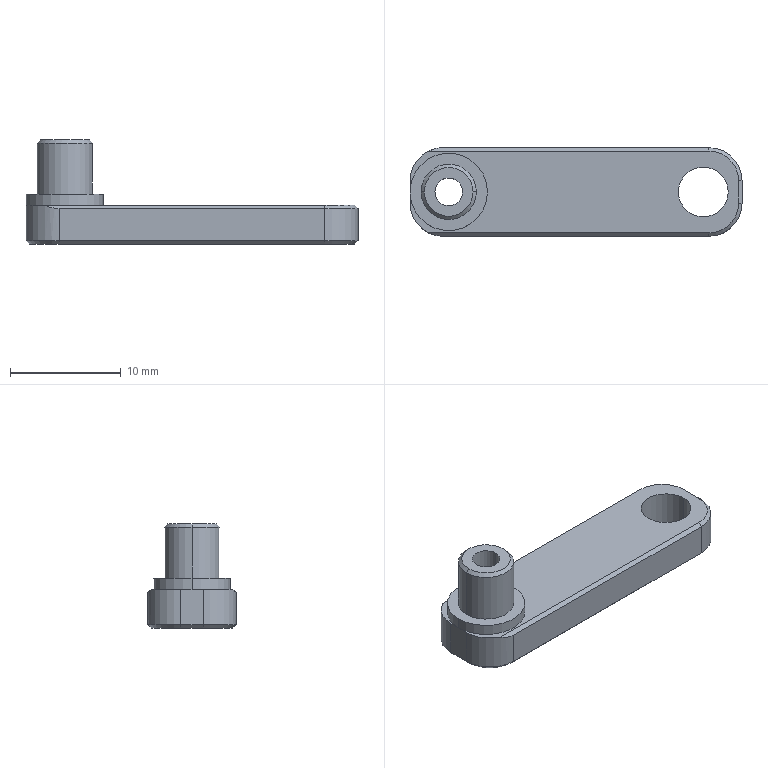Part | NX | features BREP 1 | 1 solid | 35 faces | box 30 x 8 x 9.4 mm | volume 839.286 mm3 | plane 15 | cylinder 12 | cone 8 | commonest cylinder face diameters 6 x4 2.5 x2 4.5 x2 5 x2 7 x2
STEP:
#1=CARTESIAN_POINT('',(12.,3.7,3.5));
#2=VERTEX_POINT('',#1);
#3=CARTESIAN_POINT('',(12.,4.,3.2));
#4=VERTEX_POINT('',#3);
#5=CARTESIAN_POINT('',(12.,3.7,3.5));
#6=DIRECTION('',(0.,0.7071,-0.7071));
#7=VECTOR('',#6,1000.);
#8=LINE('',#5,#7);
#9=EDGE_CURVE('',#2,#4,#8,.T.);
#10=ORIENTED_EDGE('',*,*,#9,.T.);
#11=CARTESIAN_POINT('',(-12.,4.,3.2));
#12=VERTEX_POINT('',#11);
#13=CARTESIAN_POINT('',(12.,4.,3.2));
#14=DIRECTION('',(1.,0.,0.));
#15=VECTOR('',#14,1000.);
#16=LINE('',#13,#15);
#17=EDGE_CURVE('',#12,#4,#16,.T.);
#18=ORIENTED_EDGE('',*,*,#17,.F.);
#19=CARTESIAN_POINT('',(-13.308,3.7,3.5));
#20=VERTEX_POINT('',#19);
#21=CARTESIAN_POINT('',(-13.308,3.7,3.5));
#22=CARTESIAN_POINT('',(-12.898,3.898,3.302));
#23=CARTESIAN_POINT('',(-12.455,4.,3.2));
#24=CARTESIAN_POINT('',(-12.,4.,3.2));
#25=(BOUNDED_CURVE()B_SPLINE_CURVE(3,(#21,#22,#23,#24),.UNSPECIFIED.,.F.,.F.)B_SPLINE_CURVE_WITH_KNOTS((4,4),(5.832,6.283),.UNSPECIFIED.)CURVE()GEOMETRIC_REPRESENTATION_ITEM()RATIONAL_B_SPLINE_CURVE((1.,0.9831,0.9831,1.))REPRESENTATION_ITEM(''));
#26=EDGE_CURVE('',#20,#12,#25,.T.);
#27=ORIENTED_EDGE('',*,*,#26,.F.);
#28=CARTESIAN_POINT('',(-12.,3.7,3.5));
#29=DIRECTION('',(-1.,0.,0.));
#30=VECTOR('',#29,1000.);
#31=LINE('',#28,#30);
#32=EDGE_CURVE('',#2,#20,#31,.T.);
#33=ORIENTED_EDGE('',*,*,#32,.F.);
#34=EDGE_LOOP('',(#10,#18,#27,#33));
#35=FACE_BOUND('',#34,.T.);
#36=CARTESIAN_POINT('',(0.,3.7,3.5));
#37=DIRECTION('',(0.,0.7071,0.7071));
#38=DIRECTION('',(1.,0.,0.));
#39=AXIS2_PLACEMENT_3D('',#36,#37,#38);
#40=PLANE('',#39);
#41=ADVANCED_FACE('',(#35),#40,.T.);
#42=CARTESIAN_POINT('',(14.7,1.,3.5));
#43=VERTEX_POINT('',#42);
#44=CARTESIAN_POINT('',(15.,1.,3.2));
#45=VERTEX_POINT('',#44);
#46=CARTESIAN_POINT('',(14.7,1.,3.5));
#47=DIRECTION('',(0.7071,0.,-0.7071));
#48=VECTOR('',#47,1000.);
#49=LINE('',#46,#48);
#50=EDGE_CURVE('',#43,#45,#49,.T.);
#51=ORIENTED_EDGE('',*,*,#50,.T.);
#52=CARTESIAN_POINT('',(12.,1.,3.2));
#53=DIRECTION('',(0.,0.,-1.));
#54=DIRECTION('',(1.,0.,0.));
#55=AXIS2_PLACEMENT_3D('',#52,#53,#54);
#56=CIRCLE('',#55,3.);
#57=EDGE_CURVE('',#4,#45,#56,.T.);
#58=ORIENTED_EDGE('',*,*,#57,.F.);
#59=ORIENTED_EDGE('',*,*,#9,.F.);
#60=CARTESIAN_POINT('',(12.,1.,3.5));
#61=DIRECTION('',(0.,0.,1.));
#62=DIRECTION('',(1.,0.,0.));
#63=AXIS2_PLACEMENT_3D('',#60,#61,#62);
#64=CIRCLE('',#63,2.7);
#65=EDGE_CURVE('',#43,#2,#64,.T.);
#66=ORIENTED_EDGE('',*,*,#65,.F.);
#67=EDGE_LOOP('',(#51,#58,#59,#66));
#68=FACE_BOUND('',#67,.T.);
#69=CARTESIAN_POINT('',(12.,1.,3.5));
#70=DIRECTION('',(0.,0.,-1.));
#71=DIRECTION('',(-1.,0.,0.));
#72=AXIS2_PLACEMENT_3D('',#69,#70,#71);
#73=CONICAL_SURFACE('',#72,2.7,0.7854);
#74=ADVANCED_FACE('',(#68),#73,.T.);
#75=CARTESIAN_POINT('',(14.7,-1.,3.5));
#76=VERTEX_POINT('',#75);
#77=CARTESIAN_POINT('',(15.,-1.,3.2));
#78=VERTEX_POINT('',#77);
#79=CARTESIAN_POINT('',(14.7,-1.,3.5));
#80=DIRECTION('',(0.7071,0.,-0.7071));
#81=VECTOR('',#80,1000.);
#82=LINE('',#79,#81);
#83=EDGE_CURVE('',#76,#78,#82,.T.);
#84=ORIENTED_EDGE('',*,*,#83,.T.);
#85=CARTESIAN_POINT('',(15.,-1.,3.2));
#86=DIRECTION('',(0.,-1.,0.));
#87=VECTOR('',#86,1000.);
#88=LINE('',#85,#87);
#89=EDGE_CURVE('',#45,#78,#88,.T.);
#90=ORIENTED_EDGE('',*,*,#89,.F.);
#91=ORIENTED_EDGE('',*,*,#50,.F.);
#92=CARTESIAN_POINT('',(14.7,1.,3.5));
#93=DIRECTION('',(0.,1.,0.));
#94=VECTOR('',#93,1000.);
#95=LINE('',#92,#94);
#96=EDGE_CURVE('',#76,#43,#95,.T.);
#97=ORIENTED_EDGE('',*,*,#96,.F.);
#98=EDGE_LOOP('',(#84,#90,#91,#97));
#99=FACE_BOUND('',#98,.T.);
#100=CARTESIAN_POINT('',(14.7,0.,3.5));
#101=DIRECTION('',(0.7071,0.,0.7071));
#102=DIRECTION('',(0.,-1.,0.));
#103=AXIS2_PLACEMENT_3D('',#100,#101,#102);
#104=PLANE('',#103);
#105=ADVANCED_FACE('',(#99),#104,.T.);
#106=CARTESIAN_POINT('',(12.,-3.7,3.5));
#107=VERTEX_POINT('',#106);
#108=CARTESIAN_POINT('',(12.,-4.,3.2));
#109=VERTEX_POINT('',#108);
#110=CARTESIAN_POINT('',(12.,-3.7,3.5));
#111=DIRECTION('',(0.,-0.7071,-0.7071));
#112=VECTOR('',#111,1000.);
#113=LINE('',#110,#112);
#114=EDGE_CURVE('',#107,#109,#113,.T.);
#115=ORIENTED_EDGE('',*,*,#114,.T.);
#116=CARTESIAN_POINT('',(12.,-1.,3.2));
#117=DIRECTION('',(0.,0.,-1.));
#118=DIRECTION('',(1.,0.,0.));
#119=AXIS2_PLACEMENT_3D('',#116,#117,#118);
#120=CIRCLE('',#119,3.);
#121=EDGE_CURVE('',#78,#109,#120,.T.);
#122=ORIENTED_EDGE('',*,*,#121,.F.);
#123=ORIENTED_EDGE('',*,*,#83,.F.);
#124=CARTESIAN_POINT('',(12.,-1.,3.5));
#125=DIRECTION('',(0.,0.,1.));
#126=DIRECTION('',(1.,0.,0.));
#127=AXIS2_PLACEMENT_3D('',#124,#125,#126);
#128=CIRCLE('',#127,2.7);
#129=EDGE_CURVE('',#107,#76,#128,.T.);
#130=ORIENTED_EDGE('',*,*,#129,.F.);
#131=EDGE_LOOP('',(#115,#122,#123,#130));
#132=FACE_BOUND('',#131,.T.);
#133=CARTESIAN_POINT('',(12.,-1.,3.5));
#134=DIRECTION('',(0.,0.,-1.));
#135=DIRECTION('',(-1.,0.,0.));
#136=AXIS2_PLACEMENT_3D('',#133,#134,#135);
#137=CONICAL_SURFACE('',#136,2.7,0.7854);
#138=ADVANCED_FACE('',(#132),#137,.T.);
#139=CARTESIAN_POINT('',(-12.,-4.,3.2));
#140=VERTEX_POINT('',#139);
#141=CARTESIAN_POINT('',(-13.308,-3.7,3.5));
#142=VERTEX_POINT('',#141);
#143=CARTESIAN_POINT('',(-12.,-4.,3.2));
#144=CARTESIAN_POINT('',(-12.455,-4.,3.2));
#145=CARTESIAN_POINT('',(-12.898,-3.898,3.302));
#146=CARTESIAN_POINT('',(-13.308,-3.7,3.5));
#147=(BOUNDED_CURVE()B_SPLINE_CURVE(3,(#143,#144,#145,#146),.UNSPECIFIED.,.F.,.F.)B_SPLINE_CURVE_WITH_KNOTS((4,4),(0.,0.451),.UNSPECIFIED.)CURVE()GEOMETRIC_REPRESENTATION_ITEM()RATIONAL_B_SPLINE_CURVE((1.,0.9831,0.9831,1.))REPRESENTATION_ITEM(''));
#148=EDGE_CURVE('',#140,#142,#147,.T.);
#149=ORIENTED_EDGE('',*,*,#148,.F.);
#150=CARTESIAN_POINT('',(-12.,-4.,3.2));
#151=DIRECTION('',(-1.,0.,0.));
#152=VECTOR('',#151,1000.);
#153=LINE('',#150,#152);
#154=EDGE_CURVE('',#109,#140,#153,.T.);
#155=ORIENTED_EDGE('',*,*,#154,.F.);
#156=ORIENTED_EDGE('',*,*,#114,.F.);
#157=CARTESIAN_POINT('',(12.,-3.7,3.5));
#158=DIRECTION('',(1.,0.,0.));
#159=VECTOR('',#158,1000.);
#160=LINE('',#157,#159);
#161=EDGE_CURVE('',#142,#107,#160,.T.);
#162=ORIENTED_EDGE('',*,*,#161,.F.);
#163=EDGE_LOOP('',(#149,#155,#156,#162));
#164=FACE_BOUND('',#163,.T.);
#165=CARTESIAN_POINT('',(0.,-3.7,3.5));
#166=DIRECTION('',(0.,-0.7071,0.7071));
#167=DIRECTION('',(-1.,0.,0.));
#168=AXIS2_PLACEMENT_3D('',#165,#166,#167);
#169=PLANE('',#168);
#170=ADVANCED_FACE('',(#164),#169,.T.);
#171=CARTESIAN_POINT('',(-12.,-4.,0.3));
#172=VERTEX_POINT('',#171);
#173=CARTESIAN_POINT('',(-12.,-3.7,0.));
#174=VERTEX_POINT('',#173);
#175=CARTESIAN_POINT('',(-12.,-4.,0.3));
#176=DIRECTION('',(0.,0.7071,-0.7071));
#177=VECTOR('',#176,1000.);
#178=LINE('',#175,#177);
#179=EDGE_CURVE('',#172,#174,#178,.T.);
#180=ORIENTED_EDGE('',*,*,#179,.T.);
#181=CARTESIAN_POINT('',(12.,-3.7,0.));
#182=VERTEX_POINT('',#181);
#183=CARTESIAN_POINT('',(0.,-3.7,0.));
#184=DIRECTION('',(-1.,0.,0.));
#185=VECTOR('',#184,1000.);
#186=LINE('',#183,#185);
#187=EDGE_CURVE('',#182,#174,#186,.T.);
#188=ORIENTED_EDGE('',*,*,#187,.F.);
#189=CARTESIAN_POINT('',(12.,-4.,0.3));
#190=VERTEX_POINT('',#189);
#191=CARTESIAN_POINT('',(12.,-3.7,0.));
#192=DIRECTION('',(0.,-0.7071,0.7071));
#193=VECTOR('',#192,1000.);
#194=LINE('',#191,#193);
#195=EDGE_CURVE('',#182,#190,#194,.T.);
#196=ORIENTED_EDGE('',*,*,#195,.T.);
#197=CARTESIAN_POINT('',(-15.,-4.,0.3));
#198=DIRECTION('',(1.,0.,0.));
#199=VECTOR('',#198,1000.);
#200=LINE('',#197,#199);
#201=EDGE_CURVE('',#172,#190,#200,.T.);
#202=ORIENTED_EDGE('',*,*,#201,.F.);
#203=EDGE_LOOP('',(#180,#188,#196,#202));
#204=FACE_BOUND('',#203,.T.);
#205=CARTESIAN_POINT('',(-15.,-4.,0.3));
#206=DIRECTION('',(0.,0.7071,0.7071));
#207=DIRECTION('',(1.,0.,0.));
#208=AXIS2_PLACEMENT_3D('',#205,#206,#207);
#209=PLANE('',#208);
#210=ADVANCED_FACE('',(#204),#209,.F.);
#211=CARTESIAN_POINT('',(14.7,-1.,0.));
#212=VERTEX_POINT('',#211);
#213=CARTESIAN_POINT('',(15.,-1.,0.3));
#214=VERTEX_POINT('',#213);
#215=CARTESIAN_POINT('',(14.7,-1.,0.));
#216=DIRECTION('',(0.7071,0.,0.7071));
#217=VECTOR('',#216,1000.);
#218=LINE('',#215,#217);
#219=EDGE_CURVE('',#212,#214,#218,.T.);
#220=ORIENTED_EDGE('',*,*,#219,.T.);
#221=CARTESIAN_POINT('',(12.,-1.,0.3));
#222=DIRECTION('',(0.,0.,1.));
#223=DIRECTION('',(1.,0.,0.));
#224=AXIS2_PLACEMENT_3D('',#221,#222,#223);
#225=CIRCLE('',#224,3.);
#226=EDGE_CURVE('',#190,#214,#225,.T.);
#227=ORIENTED_EDGE('',*,*,#226,.F.);
#228=ORIENTED_EDGE('',*,*,#195,.F.);
#229=CARTESIAN_POINT('',(12.,-1.,0.));
#230=DIRECTION('',(0.,0.,-1.));
#231=DIRECTION('',(1.,0.,0.));
#232=AXIS2_PLACEMENT_3D('',#229,#230,#231);
#233=CIRCLE('',#232,2.7);
#234=EDGE_CURVE('',#212,#182,#233,.T.);
#235=ORIENTED_EDGE('',*,*,#234,.F.);
#236=EDGE_LOOP('',(#220,#227,#228,#235));
#237=FACE_BOUND('',#236,.T.);
#238=CARTESIAN_POINT('',(12.,-1.,0.));
#239=DIRECTION('',(0.,0.,1.));
#240=DIRECTION('',(1.,0.,0.));
#241=AXIS2_PLACEMENT_3D('',#238,#239,#240);
#242=CONICAL_SURFACE('',#241,2.7,0.7854);
#243=ADVANCED_FACE('',(#237),#242,.T.);
#244=CARTESIAN_POINT('',(-15.,-1.,0.3));
#245=VERTEX_POINT('',#244);
#246=CARTESIAN_POINT('',(-14.7,-1.,0.));
#247=VERTEX_POINT('',#246);
#248=CARTESIAN_POINT('',(-15.,-1.,0.3));
#249=DIRECTION('',(0.7071,0.,-0.7071));
#250=VECTOR('',#249,1000.);
#251=LINE('',#248,#250);
#252=EDGE_CURVE('',#245,#247,#251,.T.);
#253=ORIENTED_EDGE('',*,*,#252,.T.);
#254=CARTESIAN_POINT('',(-12.,-1.,0.));
#255=DIRECTION('',(0.,0.,-1.));
#256=DIRECTION('',(1.,0.,0.));
#257=AXIS2_PLACEMENT_3D('',#254,#255,#256);
#258=CIRCLE('',#257,2.7);
#259=EDGE_CURVE('',#174,#247,#258,.T.);
#260=ORIENTED_EDGE('',*,*,#259,.F.);
#261=ORIENTED_EDGE('',*,*,#179,.F.);
#262=CARTESIAN_POINT('',(-12.,-1.,0.3));
#263=DIRECTION('',(0.,0.,1.));
#264=DIRECTION('',(1.,0.,0.));
#265=AXIS2_PLACEMENT_3D('',#262,#263,#264);
#266=CIRCLE('',#265,3.);
#267=EDGE_CURVE('',#245,#172,#266,.T.);
#268=ORIENTED_EDGE('',*,*,#267,.F.);
#269=EDGE_LOOP('',(#253,#260,#261,#268));
#270=FACE_BOUND('',#269,.T.);
#271=CARTESIAN_POINT('',(-12.,-1.,0.));
#272=DIRECTION('',(0.,0.,1.));
#273=DIRECTION('',(1.,0.,0.));
#274=AXIS2_PLACEMENT_3D('',#271,#272,#273);
#275=CONICAL_SURFACE('',#274,2.7,0.7854);
#276=ADVANCED_FACE('',(#270),#275,.T.);
#277=CARTESIAN_POINT('',(14.7,1.,0.));
#278=VERTEX_POINT('',#277);
#279=CARTESIAN_POINT('',(15.,1.,0.3));
#280=VERTEX_POINT('',#279);
#281=CARTESIAN_POINT('',(14.7,1.,0.));
#282=DIRECTION('',(0.7071,0.,0.7071));
#283=VECTOR('',#282,1000.);
#284=LINE('',#281,#283);
#285=EDGE_CURVE('',#278,#280,#284,.T.);
#286=ORIENTED_EDGE('',*,*,#285,.T.);
#287=CARTESIAN_POINT('',(15.,4.,0.3));
#288=DIRECTION('',(0.,1.,0.));
#289=VECTOR('',#288,1000.);
#290=LINE('',#287,#289);
#291=EDGE_CURVE('',#214,#280,#290,.T.);
#292=ORIENTED_EDGE('',*,*,#291,.F.);
#293=ORIENTED_EDGE('',*,*,#219,.F.);
#294=CARTESIAN_POINT('',(14.7,0.,0.));
#295=DIRECTION('',(0.,-1.,0.));
#296=VECTOR('',#295,1000.);
#297=LINE('',#294,#296);
#298=EDGE_CURVE('',#278,#212,#297,.T.);
#299=ORIENTED_EDGE('',*,*,#298,.F.);
#300=EDGE_LOOP('',(#286,#292,#293,#299));
#301=FACE_BOUND('',#300,.T.);
#302=CARTESIAN_POINT('',(15.,4.,0.3));
#303=DIRECTION('',(-0.7071,0.,0.7071));
#304=DIRECTION('',(0.,1.,0.));
#305=AXIS2_PLACEMENT_3D('',#302,#303,#304);
#306=PLANE('',#305);
#307=ADVANCED_FACE('',(#301),#306,.F.);
#308=CARTESIAN_POINT('',(-15.,1.,0.3));
#309=VERTEX_POINT('',#308);
#310=CARTESIAN_POINT('',(-14.7,1.,0.));
#311=VERTEX_POINT('',#310);
#312=CARTESIAN_POINT('',(-15.,1.,0.3));
#313=DIRECTION('',(0.7071,0.,-0.7071));
#314=VECTOR('',#313,1000.);
#315=LINE('',#312,#314);
#316=EDGE_CURVE('',#309,#311,#315,.T.);
#317=ORIENTED_EDGE('',*,*,#316,.T.);
#318=CARTESIAN_POINT('',(-14.7,0.,0.));
#319=DIRECTION('',(0.,1.,0.));
#320=VECTOR('',#319,1000.);
#321=LINE('',#318,#320);
#322=EDGE_CURVE('',#247,#311,#321,.T.);
#323=ORIENTED_EDGE('',*,*,#322,.F.);
#324=ORIENTED_EDGE('',*,*,#252,.F.);
#325=CARTESIAN_POINT('',(-15.,4.,0.3));
#326=DIRECTION('',(0.,-1.,0.));
#327=VECTOR('',#326,1000.);
#328=LINE('',#325,#327);
#329=EDGE_CURVE('',#309,#245,#328,.T.);
#330=ORIENTED_EDGE('',*,*,#329,.F.);
#331=EDGE_LOOP('',(#317,#323,#324,#330));
#332=FACE_BOUND('',#331,.T.);
#333=CARTESIAN_POINT('',(-15.,4.,0.3));
#334=DIRECTION('',(0.7071,0.,0.7071));
#335=DIRECTION('',(0.,-1.,0.));
#336=AXIS2_PLACEMENT_3D('',#333,#334,#335);
#337=PLANE('',#336);
#338=ADVANCED_FACE('',(#332),#337,.F.);
#339=CARTESIAN_POINT('',(12.,3.7,0.));
#340=VERTEX_POINT('',#339);
#341=CARTESIAN_POINT('',(12.,4.,0.3));
#342=VERTEX_POINT('',#341);
#343=CARTESIAN_POINT('',(12.,3.7,0.));
#344=DIRECTION('',(0.,0.7071,0.7071));
#345=VECTOR('',#344,1000.);
#346=LINE('',#343,#345);
#347=EDGE_CURVE('',#340,#342,#346,.T.);
#348=ORIENTED_EDGE('',*,*,#347,.T.);
#349=CARTESIAN_POINT('',(12.,1.,0.3));
#350=DIRECTION('',(0.,0.,1.));
#351=DIRECTION('',(1.,0.,0.));
#352=AXIS2_PLACEMENT_3D('',#349,#350,#351);
#353=CIRCLE('',#352,3.);
#354=EDGE_CURVE('',#280,#342,#353,.T.);
#355=ORIENTED_EDGE('',*,*,#354,.F.);
#356=ORIENTED_EDGE('',*,*,#285,.F.);
#357=CARTESIAN_POINT('',(12.,1.,0.));
#358=DIRECTION('',(0.,0.,-1.));
#359=DIRECTION('',(1.,0.,0.));
#360=AXIS2_PLACEMENT_3D('',#357,#358,#359);
#361=CIRCLE('',#360,2.7);
#362=EDGE_CURVE('',#340,#278,#361,.T.);
#363=ORIENTED_EDGE('',*,*,#362,.F.);
#364=EDGE_LOOP('',(#348,#355,#356,#363));
#365=FACE_BOUND('',#364,.T.);
#366=CARTESIAN_POINT('',(12.,1.,0.));
#367=DIRECTION('',(0.,0.,1.));
#368=DIRECTION('',(1.,0.,0.));
#369=AXIS2_PLACEMENT_3D('',#366,#367,#368);
#370=CONICAL_SURFACE('',#369,2.7,0.7854);
#371=ADVANCED_FACE('',(#365),#370,.T.);
#372=CARTESIAN_POINT('',(-12.,4.,0.3));
#373=VERTEX_POINT('',#372);
#374=CARTESIAN_POINT('',(-12.,3.7,0.));
#375=VERTEX_POINT('',#374);
#376=CARTESIAN_POINT('',(-12.,4.,0.3));
#377=DIRECTION('',(0.,-0.7071,-0.7071));
#378=VECTOR('',#377,1000.);
#379=LINE('',#376,#378);
#380=EDGE_CURVE('',#373,#375,#379,.T.);
#381=ORIENTED_EDGE('',*,*,#380,.T.);
#382=CARTESIAN_POINT('',(-12.,1.,0.));
#383=DIRECTION('',(0.,0.,-1.));
#384=DIRECTION('',(1.,0.,0.));
#385=AXIS2_PLACEMENT_3D('',#382,#383,#384);
#386=CIRCLE('',#385,2.7);
#387=EDGE_CURVE('',#311,#375,#386,.T.);
#388=ORIENTED_EDGE('',*,*,#387,.F.);
#389=ORIENTED_EDGE('',*,*,#316,.F.);
#390=CARTESIAN_POINT('',(-12.,1.,0.3));
#391=DIRECTION('',(0.,0.,1.));
#392=DIRECTION('',(1.,0.,0.));
#393=AXIS2_PLACEMENT_3D('',#390,#391,#392);
#394=CIRCLE('',#393,3.);
#395=EDGE_CURVE('',#373,#309,#394,.T.);
#396=ORIENTED_EDGE('',*,*,#395,.F.);
#397=EDGE_LOOP('',(#381,#388,#389,#396));
#398=FACE_BOUND('',#397,.T.);
#399=CARTESIAN_POINT('',(-12.,1.,0.));
#400=DIRECTION('',(0.,0.,1.));
#401=DIRECTION('',(1.,0.,0.));
#402=AXIS2_PLACEMENT_3D('',#399,#400,#401);
#403=CONICAL_SURFACE('',#402,2.7,0.7854);
#404=ADVANCED_FACE('',(#398),#403,.T.);
#405=ORIENTED_EDGE('',*,*,#347,.F.);
#406=CARTESIAN_POINT('',(0.,3.7,0.));
#407=DIRECTION('',(1.,0.,0.));
#408=VECTOR('',#407,1000.);
#409=LINE('',#406,#408);
#410=EDGE_CURVE('',#375,#340,#409,.T.);
#411=ORIENTED_EDGE('',*,*,#410,.F.);
#412=ORIENTED_EDGE('',*,*,#380,.F.);
#413=CARTESIAN_POINT('',(-15.,4.,0.3));
#414=DIRECTION('',(-1.,0.,0.));
#415=VECTOR('',#414,1000.);
#416=LINE('',#413,#415);
#417=EDGE_CURVE('',#342,#373,#416,.T.);
#418=ORIENTED_EDGE('',*,*,#417,.F.);
#419=EDGE_LOOP('',(#405,#411,#412,#418));
#420=FACE_BOUND('',#419,.T.);
#421=CARTESIAN_POINT('',(-15.,4.,0.3));
#422=DIRECTION('',(0.,-0.7071,0.7071));
#423=DIRECTION('',(-1.,0.,0.));
#424=AXIS2_PLACEMENT_3D('',#421,#422,#423);
#425=PLANE('',#424);
#426=ADVANCED_FACE('',(#420),#425,.F.);
#427=CARTESIAN_POINT('',(-9.3,0.,9.4));
#428=VERTEX_POINT('',#427);
#429=CARTESIAN_POINT('',(-9.,0.,9.1));
#430=VERTEX_POINT('',#429);
#431=CARTESIAN_POINT('',(-9.3,0.,9.4));
#432=DIRECTION('',(0.7071,0.,-0.7071));
#433=VECTOR('',#432,1000.);
#434=LINE('',#431,#433);
#435=EDGE_CURVE('',#428,#430,#434,.T.);
#436=ORIENTED_EDGE('',*,*,#435,.F.);
#437=CARTESIAN_POINT('',(-13.7,0.,9.4));
#438=VERTEX_POINT('',#437);
#439=CARTESIAN_POINT('',(-11.5,0.,9.4));
#440=DIRECTION('',(0.,0.,1.));
#441=DIRECTION('',(1.,0.,0.));
#442=AXIS2_PLACEMENT_3D('',#439,#440,#441);
#443=CIRCLE('',#442,2.2);
#444=EDGE_CURVE('',#438,#428,#443,.T.);
#445=ORIENTED_EDGE('',*,*,#444,.F.);
#446=CARTESIAN_POINT('',(-14.,0.,9.1));
#447=VERTEX_POINT('',#446);
#448=CARTESIAN_POINT('',(-13.7,0.,9.4));
#449=DIRECTION('',(-0.7071,0.,-0.7071));
#450=VECTOR('',#449,1000.);
#451=LINE('',#448,#450);
#452=EDGE_CURVE('',#438,#447,#451,.T.);
#453=ORIENTED_EDGE('',*,*,#452,.T.);
#454=CARTESIAN_POINT('',(-11.5,0.,9.1));
#455=DIRECTION('',(0.,0.,-1.));
#456=DIRECTION('',(1.,0.,0.));
#457=AXIS2_PLACEMENT_3D('',#454,#455,#456);
#458=CIRCLE('',#457,2.5);
#459=EDGE_CURVE('',#430,#447,#458,.T.);
#460=ORIENTED_EDGE('',*,*,#459,.F.);
#461=EDGE_LOOP('',(#436,#445,#453,#460));
#462=FACE_BOUND('',#461,.T.);
#463=CARTESIAN_POINT('',(-11.5,0.,9.4));
#464=DIRECTION('',(0.,0.,-1.));
#465=DIRECTION('',(-1.,0.,0.));
#466=AXIS2_PLACEMENT_3D('',#463,#464,#465);
#467=CONICAL_SURFACE('',#466,2.2,0.7854);
#468=ADVANCED_FACE('',(#462),#467,.T.);
#469=CARTESIAN_POINT('',(12.,4.,3.5));
#470=DIRECTION('',(0.,0.,-1.));
#471=VECTOR('',#470,1000.);
#472=LINE('',#469,#471);
#473=EDGE_CURVE('',#4,#342,#472,.T.);
#474=ORIENTED_EDGE('',*,*,#473,.F.);
#475=ORIENTED_EDGE('',*,*,#57,.T.);
#476=CARTESIAN_POINT('',(15.,1.,3.5));
#477=DIRECTION('',(0.,0.,1.));
#478=VECTOR('',#477,1000.);
#479=LINE('',#476,#478);
#480=EDGE_CURVE('',#280,#45,#479,.T.);
#481=ORIENTED_EDGE('',*,*,#480,.F.);
#482=ORIENTED_EDGE('',*,*,#354,.T.);
#483=EDGE_LOOP('',(#474,#475,#481,#482));
#484=FACE_BOUND('',#483,.T.);
#485=CARTESIAN_POINT('',(12.,1.,3.5));
#486=DIRECTION('',(0.,0.,-1.));
#487=DIRECTION('',(-1.,0.,0.));
#488=AXIS2_PLACEMENT_3D('',#485,#486,#487);
#489=CYLINDRICAL_SURFACE('',#488,3.);
#490=ADVANCED_FACE('',(#484),#489,.T.);
#491=CARTESIAN_POINT('',(15.,-1.,3.5));
#492=DIRECTION('',(0.,0.,-1.));
#493=VECTOR('',#492,1000.);
#494=LINE('',#491,#493);
#495=EDGE_CURVE('',#78,#214,#494,.T.);
#496=ORIENTED_EDGE('',*,*,#495,.F.);
#497=ORIENTED_EDGE('',*,*,#121,.T.);
#498=CARTESIAN_POINT('',(12.,-4.,3.5));
#499=DIRECTION('',(0.,0.,1.));
#500=VECTOR('',#499,1000.);
#501=LINE('',#498,#500);
#502=EDGE_CURVE('',#190,#109,#501,.T.);
#503=ORIENTED_EDGE('',*,*,#502,.F.);
#504=ORIENTED_EDGE('',*,*,#226,.T.);
#505=EDGE_LOOP('',(#496,#497,#503,#504));
#506=FACE_BOUND('',#505,.T.);
#507=CARTESIAN_POINT('',(12.,-1.,3.5));
#508=DIRECTION('',(0.,0.,-1.));
#509=DIRECTION('',(-1.,0.,0.));
#510=AXIS2_PLACEMENT_3D('',#507,#508,#509);
#511=CYLINDRICAL_SURFACE('',#510,3.);
#512=ADVANCED_FACE('',(#506),#511,.T.);
#513=CARTESIAN_POINT('',(-12.,-4.,3.5));
#514=DIRECTION('',(0.,0.,-1.));
#515=VECTOR('',#514,1000.);
#516=LINE('',#513,#515);
#517=EDGE_CURVE('',#140,#172,#516,.T.);
#518=ORIENTED_EDGE('',*,*,#517,.F.);
#519=ORIENTED_EDGE('',*,*,#148,.T.);
#520=CARTESIAN_POINT('',(-15.,-1.,3.5));
#521=VERTEX_POINT('',#520);
#522=CARTESIAN_POINT('',(-12.,-1.,3.5));
#523=DIRECTION('',(0.,0.,1.));
#524=DIRECTION('',(1.,0.,0.));
#525=AXIS2_PLACEMENT_3D('',#522,#523,#524);
#526=CIRCLE('',#525,3.);
#527=EDGE_CURVE('',#521,#142,#526,.T.);
#528=ORIENTED_EDGE('',*,*,#527,.F.);
#529=CARTESIAN_POINT('',(-15.,-1.,3.5));
#530=DIRECTION('',(0.,0.,1.));
#531=VECTOR('',#530,1000.);
#532=LINE('',#529,#531);
#533=EDGE_CURVE('',#245,#521,#532,.T.);
#534=ORIENTED_EDGE('',*,*,#533,.F.);
#535=ORIENTED_EDGE('',*,*,#267,.T.);
#536=EDGE_LOOP('',(#518,#519,#528,#534,#535));
#537=FACE_BOUND('',#536,.T.);
#538=CARTESIAN_POINT('',(-12.,-1.,3.5));
#539=DIRECTION('',(0.,0.,-1.));
#540=DIRECTION('',(-1.,0.,0.));
#541=AXIS2_PLACEMENT_3D('',#538,#539,#540);
#542=CYLINDRICAL_SURFACE('',#541,3.);
#543=ADVANCED_FACE('',(#537),#542,.T.);
#544=CARTESIAN_POINT('',(-15.,1.,3.5));
#545=VERTEX_POINT('',#544);
#546=CARTESIAN_POINT('',(-12.,1.,3.5));
#547=DIRECTION('',(0.,0.,1.));
#548=DIRECTION('',(1.,0.,0.));
#549=AXIS2_PLACEMENT_3D('',#546,#547,#548);
#550=CIRCLE('',#549,3.);
#551=EDGE_CURVE('',#20,#545,#550,.T.);
#552=ORIENTED_EDGE('',*,*,#551,.F.);
#553=ORIENTED_EDGE('',*,*,#26,.T.);
#554=CARTESIAN_POINT('',(-12.,4.,3.5));
#555=DIRECTION('',(0.,0.,1.));
#556=VECTOR('',#555,1000.);
#557=LINE('',#554,#556);
#558=EDGE_CURVE('',#373,#12,#557,.T.);
#559=ORIENTED_EDGE('',*,*,#558,.F.);
#560=ORIENTED_EDGE('',*,*,#395,.T.);
#561=CARTESIAN_POINT('',(-15.,1.,3.5));
#562=DIRECTION('',(0.,0.,-1.));
#563=VECTOR('',#562,1000.);
#564=LINE('',#561,#563);
#565=EDGE_CURVE('',#545,#309,#564,.T.);
#566=ORIENTED_EDGE('',*,*,#565,.F.);
#567=EDGE_LOOP('',(#552,#553,#559,#560,#566));
#568=FACE_BOUND('',#567,.T.);
#569=CARTESIAN_POINT('',(-12.,1.,3.5));
#570=DIRECTION('',(0.,0.,-1.));
#571=DIRECTION('',(-1.,0.,0.));
#572=AXIS2_PLACEMENT_3D('',#569,#570,#571);
#573=CYLINDRICAL_SURFACE('',#572,3.);
#574=ADVANCED_FACE('',(#568),#573,.T.);
#575=CARTESIAN_POINT('',(-12.75,0.,9.4));
#576=VERTEX_POINT('',#575);
#577=CARTESIAN_POINT('',(-12.75,0.,0.));
#578=VERTEX_POINT('',#577);
#579=CARTESIAN_POINT('',(-12.75,0.,9.4));
#580=DIRECTION('',(0.,0.,1.));
#581=VECTOR('',#580,1000.);
#582=LINE('',#579,#581);
#583=EDGE_CURVE('',#576,#578,#582,.F.);
#584=ORIENTED_EDGE('',*,*,#583,.T.);
#585=CARTESIAN_POINT('',(-10.25,0.,0.));
#586=VERTEX_POINT('',#585);
#587=CARTESIAN_POINT('',(-11.5,0.,0.));
#588=DIRECTION('',(0.,0.,1.));
#589=DIRECTION('',(1.,0.,0.));
#590=AXIS2_PLACEMENT_3D('',#587,#588,#589);
#591=CIRCLE('',#590,1.25);
#592=EDGE_CURVE('',#586,#578,#591,.T.);
#593=ORIENTED_EDGE('',*,*,#592,.F.);
#594=CARTESIAN_POINT('',(-10.25,0.,9.4));
#595=VERTEX_POINT('',#594);
#596=CARTESIAN_POINT('',(-10.25,0.,9.4));
#597=DIRECTION('',(0.,0.,1.));
#598=VECTOR('',#597,1000.);
#599=LINE('',#596,#598);
#600=EDGE_CURVE('',#595,#586,#599,.F.);
#601=ORIENTED_EDGE('',*,*,#600,.F.);
#602=CARTESIAN_POINT('',(-11.5,0.,9.4));
#603=DIRECTION('',(0.,0.,1.));
#604=DIRECTION('',(1.,0.,0.));
#605=AXIS2_PLACEMENT_3D('',#602,#603,#604);
#606=CIRCLE('',#605,1.25);
#607=EDGE_CURVE('',#595,#576,#606,.T.);
#608=ORIENTED_EDGE('',*,*,#607,.T.);
#609=EDGE_LOOP('',(#584,#593,#601,#608));
#610=FACE_BOUND('',#609,.T.);
#611=CARTESIAN_POINT('',(-11.5,0.,9.4));
#612=DIRECTION('',(0.,0.,1.));
#613=DIRECTION('',(1.,0.,0.));
#614=AXIS2_PLACEMENT_3D('',#611,#612,#613);
#615=CYLINDRICAL_SURFACE('',#614,1.25);
#616=ADVANCED_FACE('',(#610),#615,.F.);
#617=CARTESIAN_POINT('',(9.25,0.,3.5));
#618=VERTEX_POINT('',#617);
#619=CARTESIAN_POINT('',(9.25,0.,0.));
#620=VERTEX_POINT('',#619);
#621=CARTESIAN_POINT('',(9.25,0.,-11.5));
#622=DIRECTION('',(0.,0.,1.));
#623=VECTOR('',#622,1000.);
#624=LINE('',#621,#623);
#625=EDGE_CURVE('',#618,#620,#624,.F.);
#626=ORIENTED_EDGE('',*,*,#625,.T.);
#627=CARTESIAN_POINT('',(13.75,0.,0.));
#628=VERTEX_POINT('',#627);
#629=CARTESIAN_POINT('',(11.5,0.,0.));
#630=DIRECTION('',(0.,0.,1.));
#631=DIRECTION('',(1.,0.,0.));
#632=AXIS2_PLACEMENT_3D('',#629,#630,#631);
#633=CIRCLE('',#632,2.25);
#634=EDGE_CURVE('',#628,#620,#633,.T.);
#635=ORIENTED_EDGE('',*,*,#634,.F.);
#636=CARTESIAN_POINT('',(13.75,0.,3.5));
#637=VERTEX_POINT('',#636);
#638=CARTESIAN_POINT('',(13.75,0.,-11.5));
#639=DIRECTION('',(0.,0.,1.));
#640=VECTOR('',#639,1000.);
#641=LINE('',#638,#640);
#642=EDGE_CURVE('',#637,#628,#641,.F.);
#643=ORIENTED_EDGE('',*,*,#642,.F.);
#644=CARTESIAN_POINT('',(11.5,0.,3.5));
#645=DIRECTION('',(0.,0.,1.));
#646=DIRECTION('',(1.,0.,0.));
#647=AXIS2_PLACEMENT_3D('',#644,#645,#646);
#648=CIRCLE('',#647,2.25);
#649=EDGE_CURVE('',#637,#618,#648,.T.);
#650=ORIENTED_EDGE('',*,*,#649,.T.);
#651=EDGE_LOOP('',(#626,#635,#643,#650));
#652=FACE_BOUND('',#651,.T.);
#653=CARTESIAN_POINT('',(11.5,0.,-11.5));
#654=DIRECTION('',(0.,0.,1.));
#655=DIRECTION('',(1.,0.,0.));
#656=AXIS2_PLACEMENT_3D('',#653,#654,#655);
#657=CYLINDRICAL_SURFACE('',#656,2.25);
#658=ADVANCED_FACE('',(#652),#657,.F.);
#659=ORIENTED_EDGE('',*,*,#607,.F.);
#660=CARTESIAN_POINT('',(-11.5,0.,9.4));
#661=DIRECTION('',(0.,0.,1.));
#662=DIRECTION('',(1.,0.,0.));
#663=AXIS2_PLACEMENT_3D('',#660,#661,#662);
#664=CIRCLE('',#663,1.25);
#665=EDGE_CURVE('',#576,#595,#664,.T.);
#666=ORIENTED_EDGE('',*,*,#665,.F.);
#667=EDGE_LOOP('',(#659,#666));
#668=FACE_BOUND('',#667,.T.);
#669=ORIENTED_EDGE('',*,*,#444,.T.);
#670=CARTESIAN_POINT('',(-11.5,0.,9.4));
#671=DIRECTION('',(0.,0.,1.));
#672=DIRECTION('',(1.,0.,0.));
#673=AXIS2_PLACEMENT_3D('',#670,#671,#672);
#674=CIRCLE('',#673,2.2);
#675=EDGE_CURVE('',#428,#438,#674,.T.);
#676=ORIENTED_EDGE('',*,*,#675,.T.);
#677=EDGE_LOOP('',(#669,#676));
#678=FACE_BOUND('',#677,.T.);
#679=CARTESIAN_POINT('',(-11.5,0.,9.4));
#680=DIRECTION('',(0.,0.,1.));
#681=DIRECTION('',(1.,0.,0.));
#682=AXIS2_PLACEMENT_3D('',#679,#680,#681);
#683=PLANE('',#682);
#684=ADVANCED_FACE('',(#668,#678),#683,.T.);
#685=CARTESIAN_POINT('',(-9.,0.,4.5));
#686=VERTEX_POINT('',#685);
#687=CARTESIAN_POINT('',(-9.,0.,9.4));
#688=DIRECTION('',(0.,0.,-1.));
#689=VECTOR('',#688,1000.);
#690=LINE('',#687,#689);
#691=EDGE_CURVE('',#430,#686,#690,.T.);
#692=ORIENTED_EDGE('',*,*,#691,.F.);
#693=ORIENTED_EDGE('',*,*,#459,.T.);
#694=CARTESIAN_POINT('',(-14.,0.,4.5));
#695=VERTEX_POINT('',#694);
#696=CARTESIAN_POINT('',(-14.,0.,9.4));
#697=DIRECTION('',(0.,0.,-1.));
#698=VECTOR('',#697,1000.);
#699=LINE('',#696,#698);
#700=EDGE_CURVE('',#447,#695,#699,.T.);
#701=ORIENTED_EDGE('',*,*,#700,.T.);
#702=CARTESIAN_POINT('',(-11.5,0.,4.5));
#703=DIRECTION('',(0.,0.,1.));
#704=DIRECTION('',(1.,0.,0.));
#705=AXIS2_PLACEMENT_3D('',#702,#703,#704);
#706=CIRCLE('',#705,2.5);
#707=EDGE_CURVE('',#695,#686,#706,.T.);
#708=ORIENTED_EDGE('',*,*,#707,.T.);
#709=EDGE_LOOP('',(#692,#693,#701,#708));
#710=FACE_BOUND('',#709,.T.);
#711=CARTESIAN_POINT('',(-11.5,0.,9.4));
#712=DIRECTION('',(0.,0.,-1.));
#713=DIRECTION('',(-1.,0.,0.));
#714=AXIS2_PLACEMENT_3D('',#711,#712,#713);
#715=CYLINDRICAL_SURFACE('',#714,2.5);
#716=ADVANCED_FACE('',(#710),#715,.T.);
#717=CARTESIAN_POINT('',(-15.,0.,4.5));
#718=VERTEX_POINT('',#717);
#719=CARTESIAN_POINT('',(-8.,0.,4.5));
#720=VERTEX_POINT('',#719);
#721=CARTESIAN_POINT('',(-11.5,0.,4.5));
#722=DIRECTION('',(0.,0.,1.));
#723=DIRECTION('',(1.,0.,0.));
#724=AXIS2_PLACEMENT_3D('',#721,#722,#723);
#725=CIRCLE('',#724,3.5);
#726=EDGE_CURVE('',#718,#720,#725,.T.);
#727=ORIENTED_EDGE('',*,*,#726,.T.);
#728=CARTESIAN_POINT('',(-11.5,0.,4.5));
#729=DIRECTION('',(0.,0.,1.));
#730=DIRECTION('',(1.,0.,0.));
#731=AXIS2_PLACEMENT_3D('',#728,#729,#730);
#732=CIRCLE('',#731,3.5);
#733=EDGE_CURVE('',#720,#718,#732,.T.);
#734=ORIENTED_EDGE('',*,*,#733,.T.);
#735=EDGE_LOOP('',(#727,#734));
#736=FACE_BOUND('',#735,.T.);
#737=ORIENTED_EDGE('',*,*,#707,.F.);
#738=CARTESIAN_POINT('',(-11.5,0.,4.5));
#739=DIRECTION('',(0.,0.,1.));
#740=DIRECTION('',(1.,0.,0.));
#741=AXIS2_PLACEMENT_3D('',#738,#739,#740);
#742=CIRCLE('',#741,2.5);
#743=EDGE_CURVE('',#686,#695,#742,.T.);
#744=ORIENTED_EDGE('',*,*,#743,.F.);
#745=EDGE_LOOP('',(#737,#744));
#746=FACE_BOUND('',#745,.T.);
#747=CARTESIAN_POINT('',(-11.5,0.,4.5));
#748=DIRECTION('',(0.,0.,1.));
#749=DIRECTION('',(1.,0.,0.));
#750=AXIS2_PLACEMENT_3D('',#747,#748,#749);
#751=PLANE('',#750);
#752=ADVANCED_FACE('',(#736,#746),#751,.T.);
#753=CARTESIAN_POINT('',(-8.,0.,3.5));
#754=VERTEX_POINT('',#753);
#755=CARTESIAN_POINT('',(-8.,0.,4.5));
#756=DIRECTION('',(0.,0.,-1.));
#757=VECTOR('',#756,1000.);
#758=LINE('',#755,#757);
#759=EDGE_CURVE('',#720,#754,#758,.T.);
#760=ORIENTED_EDGE('',*,*,#759,.F.);
#761=ORIENTED_EDGE('',*,*,#726,.F.);
#762=CARTESIAN_POINT('',(-15.,0.,3.5));
#763=VERTEX_POINT('',#762);
#764=CARTESIAN_POINT('',(-15.,0.,4.5));
#765=DIRECTION('',(0.,0.,-1.));
#766=VECTOR('',#765,1000.);
#767=LINE('',#764,#766);
#768=EDGE_CURVE('',#718,#763,#767,.T.);
#769=ORIENTED_EDGE('',*,*,#768,.T.);
#770=CARTESIAN_POINT('',(-11.5,0.,3.5));
#771=DIRECTION('',(0.,0.,1.));
#772=DIRECTION('',(1.,0.,0.));
#773=AXIS2_PLACEMENT_3D('',#770,#771,#772);
#774=CIRCLE('',#773,3.5);
#775=EDGE_CURVE('',#763,#754,#774,.T.);
#776=ORIENTED_EDGE('',*,*,#775,.T.);
#777=EDGE_LOOP('',(#760,#761,#769,#776));
#778=FACE_BOUND('',#777,.T.);
#779=CARTESIAN_POINT('',(-11.5,0.,4.5));
#780=DIRECTION('',(0.,0.,-1.));
#781=DIRECTION('',(-1.,0.,0.));
#782=AXIS2_PLACEMENT_3D('',#779,#780,#781);
#783=CYLINDRICAL_SURFACE('',#782,3.5);
#784=ADVANCED_FACE('',(#778),#783,.T.);
#785=ORIENTED_EDGE('',*,*,#634,.T.);
#786=CARTESIAN_POINT('',(11.5,0.,0.));
#787=DIRECTION('',(0.,0.,1.));
#788=DIRECTION('',(1.,0.,0.));
#789=AXIS2_PLACEMENT_3D('',#786,#787,#788);
#790=CIRCLE('',#789,2.25);
#791=EDGE_CURVE('',#620,#628,#790,.T.);
#792=ORIENTED_EDGE('',*,*,#791,.T.);
#793=EDGE_LOOP('',(#785,#792));
#794=FACE_BOUND('',#793,.T.);
#795=ORIENTED_EDGE('',*,*,#592,.T.);
#796=CARTESIAN_POINT('',(-11.5,0.,0.));
#797=DIRECTION('',(0.,0.,1.));
#798=DIRECTION('',(1.,0.,0.));
#799=AXIS2_PLACEMENT_3D('',#796,#797,#798);
#800=CIRCLE('',#799,1.25);
#801=EDGE_CURVE('',#578,#586,#800,.T.);
#802=ORIENTED_EDGE('',*,*,#801,.T.);
#803=EDGE_LOOP('',(#795,#802));
#804=FACE_BOUND('',#803,.T.);
#805=ORIENTED_EDGE('',*,*,#234,.T.);
#806=ORIENTED_EDGE('',*,*,#187,.T.);
#807=ORIENTED_EDGE('',*,*,#259,.T.);
#808=ORIENTED_EDGE('',*,*,#322,.T.);
#809=ORIENTED_EDGE('',*,*,#387,.T.);
#810=ORIENTED_EDGE('',*,*,#410,.T.);
#811=ORIENTED_EDGE('',*,*,#362,.T.);
#812=ORIENTED_EDGE('',*,*,#298,.T.);
#813=EDGE_LOOP('',(#805,#806,#807,#808,#809,#810,#811,#812));
#814=FACE_BOUND('',#813,.T.);
#815=CARTESIAN_POINT('',(0.,0.,0.));
#816=DIRECTION('',(0.,0.,1.));
#817=DIRECTION('',(1.,0.,0.));
#818=AXIS2_PLACEMENT_3D('',#815,#816,#817);
#819=PLANE('',#818);
#820=ADVANCED_FACE('',(#794,#804,#814),#819,.F.);
#821=ORIENTED_EDGE('',*,*,#65,.T.);
#822=ORIENTED_EDGE('',*,*,#32,.T.);
#823=ORIENTED_EDGE('',*,*,#551,.T.);
#824=CARTESIAN_POINT('',(-15.,4.,3.5));
#825=DIRECTION('',(0.,-1.,0.));
#826=VECTOR('',#825,1000.);
#827=LINE('',#824,#826);
#828=EDGE_CURVE('',#545,#763,#827,.T.);
#829=ORIENTED_EDGE('',*,*,#828,.T.);
#830=CARTESIAN_POINT('',(-11.5,0.,3.5));
#831=DIRECTION('',(0.,0.,1.));
#832=DIRECTION('',(1.,0.,0.));
#833=AXIS2_PLACEMENT_3D('',#830,#831,#832);
#834=CIRCLE('',#833,3.5);
#835=EDGE_CURVE('',#754,#763,#834,.T.);
#836=ORIENTED_EDGE('',*,*,#835,.F.);
#837=ORIENTED_EDGE('',*,*,#775,.F.);
#838=CARTESIAN_POINT('',(-15.,4.,3.5));
#839=DIRECTION('',(0.,-1.,0.));
#840=VECTOR('',#839,1000.);
#841=LINE('',#838,#840);
#842=EDGE_CURVE('',#763,#521,#841,.T.);
#843=ORIENTED_EDGE('',*,*,#842,.T.);
#844=ORIENTED_EDGE('',*,*,#527,.T.);
#845=ORIENTED_EDGE('',*,*,#161,.T.);
#846=ORIENTED_EDGE('',*,*,#129,.T.);
#847=ORIENTED_EDGE('',*,*,#96,.T.);
#848=EDGE_LOOP('',(#821,#822,#823,#829,#836,#837,#843,#844,#845,#846,#847));
#849=FACE_BOUND('',#848,.T.);
#850=ORIENTED_EDGE('',*,*,#649,.F.);
#851=CARTESIAN_POINT('',(11.5,0.,3.5));
#852=DIRECTION('',(0.,0.,1.));
#853=DIRECTION('',(1.,0.,0.));
#854=AXIS2_PLACEMENT_3D('',#851,#852,#853);
#855=CIRCLE('',#854,2.25);
#856=EDGE_CURVE('',#618,#637,#855,.T.);
#857=ORIENTED_EDGE('',*,*,#856,.F.);
#858=EDGE_LOOP('',(#850,#857));
#859=FACE_BOUND('',#858,.T.);
#860=CARTESIAN_POINT('',(0.,0.,3.5));
#861=DIRECTION('',(0.,0.,1.));
#862=DIRECTION('',(1.,0.,0.));
#863=AXIS2_PLACEMENT_3D('',#860,#861,#862);
#864=PLANE('',#863);
#865=ADVANCED_FACE('',(#849,#859),#864,.T.);
#866=ORIENTED_EDGE('',*,*,#502,.T.);
#867=ORIENTED_EDGE('',*,*,#154,.T.);
#868=ORIENTED_EDGE('',*,*,#517,.T.);
#869=ORIENTED_EDGE('',*,*,#201,.T.);
#870=EDGE_LOOP('',(#866,#867,#868,#869));
#871=FACE_BOUND('',#870,.T.);
#872=CARTESIAN_POINT('',(-15.,-4.,3.5));
#873=DIRECTION('',(0.,1.,0.));
#874=DIRECTION('',(0.,0.,1.));
#875=AXIS2_PLACEMENT_3D('',#872,#873,#874);
#876=PLANE('',#875);
#877=ADVANCED_FACE('',(#871),#876,.F.);
#878=ORIENTED_EDGE('',*,*,#565,.T.);
#879=ORIENTED_EDGE('',*,*,#329,.T.);
#880=ORIENTED_EDGE('',*,*,#533,.T.);
#881=ORIENTED_EDGE('',*,*,#842,.F.);
#882=ORIENTED_EDGE('',*,*,#828,.F.);
#883=EDGE_LOOP('',(#878,#879,#880,#881,#882));
#884=FACE_BOUND('',#883,.T.);
#885=CARTESIAN_POINT('',(-15.,4.,3.5));
#886=DIRECTION('',(1.,0.,0.));
#887=DIRECTION('',(0.,0.,-1.));
#888=AXIS2_PLACEMENT_3D('',#885,#886,#887);
#889=PLANE('',#888);
#890=ADVANCED_FACE('',(#884),#889,.F.);
#891=ORIENTED_EDGE('',*,*,#558,.T.);
#892=ORIENTED_EDGE('',*,*,#17,.T.);
#893=ORIENTED_EDGE('',*,*,#473,.T.);
#894=ORIENTED_EDGE('',*,*,#417,.T.);
#895=EDGE_LOOP('',(#891,#892,#893,#894));
#896=FACE_BOUND('',#895,.T.);
#897=CARTESIAN_POINT('',(-15.,4.,3.5));
#898=DIRECTION('',(0.,-1.,0.));
#899=DIRECTION('',(0.,0.,-1.));
#900=AXIS2_PLACEMENT_3D('',#897,#898,#899);
#901=PLANE('',#900);
#902=ADVANCED_FACE('',(#896),#901,.F.);
#903=ORIENTED_EDGE('',*,*,#480,.T.);
#904=ORIENTED_EDGE('',*,*,#89,.T.);
#905=ORIENTED_EDGE('',*,*,#495,.T.);
#906=ORIENTED_EDGE('',*,*,#291,.T.);
#907=EDGE_LOOP('',(#903,#904,#905,#906));
#908=FACE_BOUND('',#907,.T.);
#909=CARTESIAN_POINT('',(15.,4.,3.5));
#910=DIRECTION('',(-1.,0.,0.));
#911=DIRECTION('',(0.,0.,1.));
#912=AXIS2_PLACEMENT_3D('',#909,#910,#911);
#913=PLANE('',#912);
#914=ADVANCED_FACE('',(#908),#913,.F.);
#915=ORIENTED_EDGE('',*,*,#733,.F.);
#916=ORIENTED_EDGE('',*,*,#759,.T.);
#917=ORIENTED_EDGE('',*,*,#835,.T.);
#918=ORIENTED_EDGE('',*,*,#768,.F.);
#919=EDGE_LOOP('',(#915,#916,#917,#918));
#920=FACE_BOUND('',#919,.T.);
#921=CARTESIAN_POINT('',(-11.5,0.,4.5));
#922=DIRECTION('',(0.,0.,-1.));
#923=DIRECTION('',(-1.,0.,0.));
#924=AXIS2_PLACEMENT_3D('',#921,#922,#923);
#925=CYLINDRICAL_SURFACE('',#924,3.5);
#926=ADVANCED_FACE('',(#920),#925,.T.);
#927=CARTESIAN_POINT('',(-11.5,0.,9.1));
#928=DIRECTION('',(0.,0.,-1.));
#929=DIRECTION('',(1.,0.,0.));
#930=AXIS2_PLACEMENT_3D('',#927,#928,#929);
#931=CIRCLE('',#930,2.5);
#932=EDGE_CURVE('',#447,#430,#931,.T.);
#933=ORIENTED_EDGE('',*,*,#932,.T.);
#934=ORIENTED_EDGE('',*,*,#691,.T.);
#935=ORIENTED_EDGE('',*,*,#743,.T.);
#936=ORIENTED_EDGE('',*,*,#700,.F.);
#937=EDGE_LOOP('',(#933,#934,#935,#936));
#938=FACE_BOUND('',#937,.T.);
#939=CARTESIAN_POINT('',(-11.5,0.,9.4));
#940=DIRECTION('',(0.,0.,-1.));
#941=DIRECTION('',(-1.,0.,0.));
#942=AXIS2_PLACEMENT_3D('',#939,#940,#941);
#943=CYLINDRICAL_SURFACE('',#942,2.5);
#944=ADVANCED_FACE('',(#938),#943,.T.);
#945=ORIENTED_EDGE('',*,*,#791,.F.);
#946=ORIENTED_EDGE('',*,*,#625,.F.);
#947=ORIENTED_EDGE('',*,*,#856,.T.);
#948=ORIENTED_EDGE('',*,*,#642,.T.);
#949=EDGE_LOOP('',(#945,#946,#947,#948));
#950=FACE_BOUND('',#949,.T.);
#951=CARTESIAN_POINT('',(11.5,0.,-11.5));
#952=DIRECTION('',(0.,0.,1.));
#953=DIRECTION('',(1.,0.,0.));
#954=AXIS2_PLACEMENT_3D('',#951,#952,#953);
#955=CYLINDRICAL_SURFACE('',#954,2.25);
#956=ADVANCED_FACE('',(#950),#955,.F.);
#957=ORIENTED_EDGE('',*,*,#801,.F.);
#958=ORIENTED_EDGE('',*,*,#583,.F.);
#959=ORIENTED_EDGE('',*,*,#665,.T.);
#960=ORIENTED_EDGE('',*,*,#600,.T.);
#961=EDGE_LOOP('',(#957,#958,#959,#960));
#962=FACE_BOUND('',#961,.T.);
#963=CARTESIAN_POINT('',(-11.5,0.,9.4));
#964=DIRECTION('',(0.,0.,1.));
#965=DIRECTION('',(1.,0.,0.));
#966=AXIS2_PLACEMENT_3D('',#963,#964,#965);
#967=CYLINDRICAL_SURFACE('',#966,1.25);
#968=ADVANCED_FACE('',(#962),#967,.F.);
#969=ORIENTED_EDGE('',*,*,#675,.F.);
#970=ORIENTED_EDGE('',*,*,#435,.T.);
#971=ORIENTED_EDGE('',*,*,#932,.F.);
#972=ORIENTED_EDGE('',*,*,#452,.F.);
#973=EDGE_LOOP('',(#969,#970,#971,#972));
#974=FACE_BOUND('',#973,.T.);
#975=CARTESIAN_POINT('',(-11.5,0.,9.4));
#976=DIRECTION('',(0.,0.,-1.));
#977=DIRECTION('',(-1.,0.,0.));
#978=AXIS2_PLACEMENT_3D('',#975,#976,#977);
#979=CONICAL_SURFACE('',#978,2.2,0.7854);
#980=ADVANCED_FACE('',(#974),#979,.T.);
#981=CLOSED_SHELL('',(#41,#74,#105,#138,#170,#210,#243,#276,#307,#338,#371,#404,#426,#468,#490,#512,#543,#574,#616,#658,#684,#716,#752,#784,#820,#865,#877,#890,#902,#914,#926,#944,#956,#968,#980));
#982=MANIFOLD_SOLID_BREP('',#981);
#983=(LENGTH_UNIT()NAMED_UNIT(*)SI_UNIT(.MILLI.,.METRE.));
#984=UNCERTAINTY_MEASURE_WITH_UNIT(LENGTH_MEASURE(0.00001),#983,'','');
#985=(NAMED_UNIT(*)PLANE_ANGLE_UNIT()SI_UNIT($,.RADIAN.));
#986=(NAMED_UNIT(*)SI_UNIT($,.STERADIAN.)SOLID_ANGLE_UNIT());
#987=(GEOMETRIC_REPRESENTATION_CONTEXT(3)GLOBAL_UNCERTAINTY_ASSIGNED_CONTEXT((#984))GLOBAL_UNIT_ASSIGNED_CONTEXT((#983,#985,#986))REPRESENTATION_CONTEXT('',''));
#988=ADVANCED_BREP_SHAPE_REPRESENTATION('',(#982),#987);